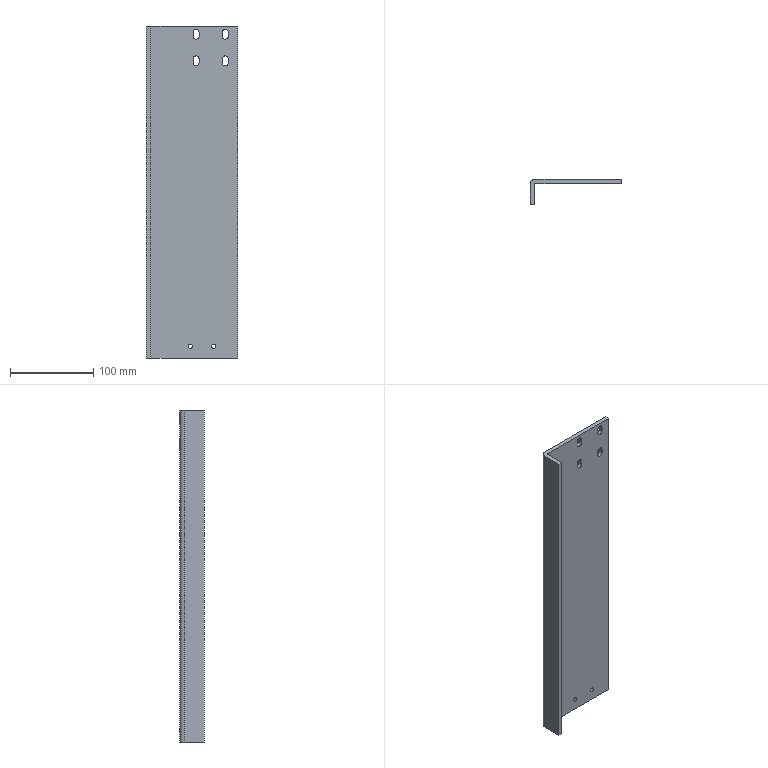Part | STEP file | Hydraulic Cylinder Bracket | 1 solid | 34 faces | box 110 x 30 x 400 mm | volume 265743 mm3 | cylinder 18 | plane 16 | commonest cylinder face diameters 7 x12 5.2 x4 1 x1 11 x1
STEP:
#1=CARTESIAN_POINT('',(81.,20.,16.6));
#2=VERTEX_POINT('',#1);
#3=CARTESIAN_POINT('',(81.,20.,11.4));
#4=VERTEX_POINT('',#3);
#5=CARTESIAN_POINT('',(81.,20.,14.));
#6=DIRECTION('',(0.,-1.,0.));
#7=DIRECTION('',(0.,0.,-1.));
#8=AXIS2_PLACEMENT_3D('',#5,#6,#7);
#9=CIRCLE('',#8,2.6);
#10=EDGE_CURVE('',#2,#4,#9,.T.);
#11=ORIENTED_EDGE('',*,*,#10,.F.);
#12=CARTESIAN_POINT('',(81.,15.,16.6));
#13=VERTEX_POINT('',#12);
#14=CARTESIAN_POINT('',(81.,20.,16.6));
#15=DIRECTION('',(0.,-1.,0.));
#16=VECTOR('',#15,1000.);
#17=LINE('',#14,#16);
#18=EDGE_CURVE('',#2,#13,#17,.T.);
#19=ORIENTED_EDGE('',*,*,#18,.T.);
#20=CARTESIAN_POINT('',(81.,15.,11.4));
#21=VERTEX_POINT('',#20);
#22=CARTESIAN_POINT('',(81.,15.,14.));
#23=DIRECTION('',(0.,1.,0.));
#24=DIRECTION('',(0.,0.,-1.));
#25=AXIS2_PLACEMENT_3D('',#22,#23,#24);
#26=CIRCLE('',#25,2.6);
#27=EDGE_CURVE('',#21,#13,#26,.T.);
#28=ORIENTED_EDGE('',*,*,#27,.F.);
#29=CARTESIAN_POINT('',(81.,20.,11.4));
#30=DIRECTION('',(0.,-1.,0.));
#31=VECTOR('',#30,1000.);
#32=LINE('',#29,#31);
#33=EDGE_CURVE('',#4,#21,#32,.T.);
#34=ORIENTED_EDGE('',*,*,#33,.F.);
#35=EDGE_LOOP('',(#11,#19,#28,#34));
#36=FACE_OUTER_BOUND('',#35,.T.);
#37=CARTESIAN_POINT('',(81.,20.,14.));
#38=DIRECTION('',(0.,-1.,0.));
#39=DIRECTION('',(0.,0.,-1.));
#40=AXIS2_PLACEMENT_3D('',#37,#38,#39);
#41=CYLINDRICAL_SURFACE('',#40,2.6);
#42=ADVANCED_FACE('',(#36),#41,.F.);
#43=CARTESIAN_POINT('',(53.,20.,16.6));
#44=VERTEX_POINT('',#43);
#45=CARTESIAN_POINT('',(53.,20.,11.4));
#46=VERTEX_POINT('',#45);
#47=CARTESIAN_POINT('',(53.,20.,14.));
#48=DIRECTION('',(0.,-1.,0.));
#49=DIRECTION('',(0.,0.,-1.));
#50=AXIS2_PLACEMENT_3D('',#47,#48,#49);
#51=CIRCLE('',#50,2.6);
#52=EDGE_CURVE('',#44,#46,#51,.T.);
#53=ORIENTED_EDGE('',*,*,#52,.F.);
#54=CARTESIAN_POINT('',(53.,15.,16.6));
#55=VERTEX_POINT('',#54);
#56=CARTESIAN_POINT('',(53.,20.,16.6));
#57=DIRECTION('',(0.,-1.,0.));
#58=VECTOR('',#57,1000.);
#59=LINE('',#56,#58);
#60=EDGE_CURVE('',#44,#55,#59,.T.);
#61=ORIENTED_EDGE('',*,*,#60,.T.);
#62=CARTESIAN_POINT('',(53.,15.,11.4));
#63=VERTEX_POINT('',#62);
#64=CARTESIAN_POINT('',(53.,15.,14.));
#65=DIRECTION('',(0.,1.,0.));
#66=DIRECTION('',(0.,0.,-1.));
#67=AXIS2_PLACEMENT_3D('',#64,#65,#66);
#68=CIRCLE('',#67,2.6);
#69=EDGE_CURVE('',#63,#55,#68,.T.);
#70=ORIENTED_EDGE('',*,*,#69,.F.);
#71=CARTESIAN_POINT('',(53.,20.,11.4));
#72=DIRECTION('',(0.,-1.,0.));
#73=VECTOR('',#72,1000.);
#74=LINE('',#71,#73);
#75=EDGE_CURVE('',#46,#63,#74,.T.);
#76=ORIENTED_EDGE('',*,*,#75,.F.);
#77=EDGE_LOOP('',(#53,#61,#70,#76));
#78=FACE_OUTER_BOUND('',#77,.T.);
#79=CARTESIAN_POINT('',(53.,20.,14.));
#80=DIRECTION('',(0.,-1.,0.));
#81=DIRECTION('',(0.,0.,-1.));
#82=AXIS2_PLACEMENT_3D('',#79,#80,#81);
#83=CYLINDRICAL_SURFACE('',#82,2.6);
#84=ADVANCED_FACE('',(#78),#83,.F.);
#85=CARTESIAN_POINT('',(95.,20.,384.));
#86=VERTEX_POINT('',#85);
#87=CARTESIAN_POINT('',(98.5,20.,387.5));
#88=VERTEX_POINT('',#87);
#89=CARTESIAN_POINT('',(95.,20.,387.5));
#90=DIRECTION('',(0.,-1.,0.));
#91=DIRECTION('',(0.,0.,-1.));
#92=AXIS2_PLACEMENT_3D('',#89,#90,#91);
#93=CIRCLE('',#92,3.5);
#94=EDGE_CURVE('',#86,#88,#93,.T.);
#95=ORIENTED_EDGE('',*,*,#94,.F.);
#96=CARTESIAN_POINT('',(95.,15.,384.));
#97=VERTEX_POINT('',#96);
#98=CARTESIAN_POINT('',(95.,25.,384.));
#99=DIRECTION('',(0.,-1.,0.));
#100=VECTOR('',#99,1000.);
#101=LINE('',#98,#100);
#102=EDGE_CURVE('',#86,#97,#101,.T.);
#103=ORIENTED_EDGE('',*,*,#102,.T.);
#104=CARTESIAN_POINT('',(98.5,15.,387.5));
#105=VERTEX_POINT('',#104);
#106=CARTESIAN_POINT('',(95.,15.,387.5));
#107=DIRECTION('',(0.,1.,0.));
#108=DIRECTION('',(0.,0.,-1.));
#109=AXIS2_PLACEMENT_3D('',#106,#107,#108);
#110=CIRCLE('',#109,3.5);
#111=EDGE_CURVE('',#105,#97,#110,.T.);
#112=ORIENTED_EDGE('',*,*,#111,.F.);
#113=CARTESIAN_POINT('',(98.5,25.,387.5));
#114=DIRECTION('',(0.,1.,0.));
#115=VECTOR('',#114,1000.);
#116=LINE('',#113,#115);
#117=EDGE_CURVE('',#105,#88,#116,.T.);
#118=ORIENTED_EDGE('',*,*,#117,.T.);
#119=EDGE_LOOP('',(#95,#103,#112,#118));
#120=FACE_OUTER_BOUND('',#119,.T.);
#121=CARTESIAN_POINT('',(95.,25.,387.5));
#122=DIRECTION('',(0.,-1.,0.));
#123=DIRECTION('',(0.,0.,-1.));
#124=AXIS2_PLACEMENT_3D('',#121,#122,#123);
#125=CYLINDRICAL_SURFACE('',#124,3.5);
#126=ADVANCED_FACE('',(#120),#125,.F.);
#127=CARTESIAN_POINT('',(60.,20.,384.));
#128=VERTEX_POINT('',#127);
#129=CARTESIAN_POINT('',(63.5,20.,387.5));
#130=VERTEX_POINT('',#129);
#131=CARTESIAN_POINT('',(60.,20.,387.5));
#132=DIRECTION('',(0.,-1.,0.));
#133=DIRECTION('',(0.,0.,-1.));
#134=AXIS2_PLACEMENT_3D('',#131,#132,#133);
#135=CIRCLE('',#134,3.5);
#136=EDGE_CURVE('',#128,#130,#135,.T.);
#137=ORIENTED_EDGE('',*,*,#136,.F.);
#138=CARTESIAN_POINT('',(60.,15.,384.));
#139=VERTEX_POINT('',#138);
#140=CARTESIAN_POINT('',(60.,25.,384.));
#141=DIRECTION('',(0.,-1.,0.));
#142=VECTOR('',#141,1000.);
#143=LINE('',#140,#142);
#144=EDGE_CURVE('',#128,#139,#143,.T.);
#145=ORIENTED_EDGE('',*,*,#144,.T.);
#146=CARTESIAN_POINT('',(63.5,15.,387.5));
#147=VERTEX_POINT('',#146);
#148=CARTESIAN_POINT('',(60.,15.,387.5));
#149=DIRECTION('',(0.,1.,0.));
#150=DIRECTION('',(0.,0.,-1.));
#151=AXIS2_PLACEMENT_3D('',#148,#149,#150);
#152=CIRCLE('',#151,3.5);
#153=EDGE_CURVE('',#147,#139,#152,.T.);
#154=ORIENTED_EDGE('',*,*,#153,.F.);
#155=CARTESIAN_POINT('',(63.5,25.,387.5));
#156=DIRECTION('',(0.,1.,0.));
#157=VECTOR('',#156,1000.);
#158=LINE('',#155,#157);
#159=EDGE_CURVE('',#147,#130,#158,.T.);
#160=ORIENTED_EDGE('',*,*,#159,.T.);
#161=EDGE_LOOP('',(#137,#145,#154,#160));
#162=FACE_OUTER_BOUND('',#161,.T.);
#163=CARTESIAN_POINT('',(60.,25.,387.5));
#164=DIRECTION('',(0.,-1.,0.));
#165=DIRECTION('',(0.,0.,-1.));
#166=AXIS2_PLACEMENT_3D('',#163,#164,#165);
#167=CYLINDRICAL_SURFACE('',#166,3.5);
#168=ADVANCED_FACE('',(#162),#167,.F.);
#169=CARTESIAN_POINT('',(60.,20.,352.));
#170=VERTEX_POINT('',#169);
#171=CARTESIAN_POINT('',(63.5,20.,355.5));
#172=VERTEX_POINT('',#171);
#173=CARTESIAN_POINT('',(60.,20.,355.5));
#174=DIRECTION('',(0.,-1.,0.));
#175=DIRECTION('',(0.,0.,-1.));
#176=AXIS2_PLACEMENT_3D('',#173,#174,#175);
#177=CIRCLE('',#176,3.5);
#178=EDGE_CURVE('',#170,#172,#177,.T.);
#179=ORIENTED_EDGE('',*,*,#178,.F.);
#180=CARTESIAN_POINT('',(60.,15.,352.));
#181=VERTEX_POINT('',#180);
#182=CARTESIAN_POINT('',(60.,25.,352.));
#183=DIRECTION('',(0.,-1.,0.));
#184=VECTOR('',#183,1000.);
#185=LINE('',#182,#184);
#186=EDGE_CURVE('',#170,#181,#185,.T.);
#187=ORIENTED_EDGE('',*,*,#186,.T.);
#188=CARTESIAN_POINT('',(63.5,15.,355.5));
#189=VERTEX_POINT('',#188);
#190=CARTESIAN_POINT('',(60.,15.,355.5));
#191=DIRECTION('',(0.,1.,0.));
#192=DIRECTION('',(0.,0.,-1.));
#193=AXIS2_PLACEMENT_3D('',#190,#191,#192);
#194=CIRCLE('',#193,3.5);
#195=EDGE_CURVE('',#189,#181,#194,.T.);
#196=ORIENTED_EDGE('',*,*,#195,.F.);
#197=CARTESIAN_POINT('',(63.5,25.,355.5));
#198=DIRECTION('',(0.,1.,0.));
#199=VECTOR('',#198,1000.);
#200=LINE('',#197,#199);
#201=EDGE_CURVE('',#189,#172,#200,.T.);
#202=ORIENTED_EDGE('',*,*,#201,.T.);
#203=EDGE_LOOP('',(#179,#187,#196,#202));
#204=FACE_OUTER_BOUND('',#203,.T.);
#205=CARTESIAN_POINT('',(60.,25.,355.5));
#206=DIRECTION('',(0.,-1.,0.));
#207=DIRECTION('',(0.,0.,-1.));
#208=AXIS2_PLACEMENT_3D('',#205,#206,#207);
#209=CYLINDRICAL_SURFACE('',#208,3.5);
#210=ADVANCED_FACE('',(#204),#209,.F.);
#211=CARTESIAN_POINT('',(95.,20.,352.));
#212=VERTEX_POINT('',#211);
#213=CARTESIAN_POINT('',(98.5,20.,355.5));
#214=VERTEX_POINT('',#213);
#215=CARTESIAN_POINT('',(95.,20.,355.5));
#216=DIRECTION('',(0.,-1.,0.));
#217=DIRECTION('',(0.,0.,-1.));
#218=AXIS2_PLACEMENT_3D('',#215,#216,#217);
#219=CIRCLE('',#218,3.5);
#220=EDGE_CURVE('',#212,#214,#219,.T.);
#221=ORIENTED_EDGE('',*,*,#220,.F.);
#222=CARTESIAN_POINT('',(95.,15.,352.));
#223=VERTEX_POINT('',#222);
#224=CARTESIAN_POINT('',(95.,25.,352.));
#225=DIRECTION('',(0.,-1.,0.));
#226=VECTOR('',#225,1000.);
#227=LINE('',#224,#226);
#228=EDGE_CURVE('',#212,#223,#227,.T.);
#229=ORIENTED_EDGE('',*,*,#228,.T.);
#230=CARTESIAN_POINT('',(98.5,15.,355.5));
#231=VERTEX_POINT('',#230);
#232=CARTESIAN_POINT('',(95.,15.,355.5));
#233=DIRECTION('',(0.,1.,0.));
#234=DIRECTION('',(0.,0.,-1.));
#235=AXIS2_PLACEMENT_3D('',#232,#233,#234);
#236=CIRCLE('',#235,3.5);
#237=EDGE_CURVE('',#231,#223,#236,.T.);
#238=ORIENTED_EDGE('',*,*,#237,.F.);
#239=CARTESIAN_POINT('',(98.5,25.,355.5));
#240=DIRECTION('',(0.,1.,0.));
#241=VECTOR('',#240,1000.);
#242=LINE('',#239,#241);
#243=EDGE_CURVE('',#231,#214,#242,.T.);
#244=ORIENTED_EDGE('',*,*,#243,.T.);
#245=EDGE_LOOP('',(#221,#229,#238,#244));
#246=FACE_OUTER_BOUND('',#245,.T.);
#247=CARTESIAN_POINT('',(95.,25.,355.5));
#248=DIRECTION('',(0.,-1.,0.));
#249=DIRECTION('',(0.,0.,-1.));
#250=AXIS2_PLACEMENT_3D('',#247,#248,#249);
#251=CYLINDRICAL_SURFACE('',#250,3.5);
#252=ADVANCED_FACE('',(#246),#251,.F.);
#253=CARTESIAN_POINT('',(5.5,20.,400.));
#254=VERTEX_POINT('',#253);
#255=CARTESIAN_POINT('',(110.,20.,400.));
#256=VERTEX_POINT('',#255);
#257=CARTESIAN_POINT('',(0.,20.,400.));
#258=DIRECTION('',(1.,0.,0.));
#259=VECTOR('',#258,1000.);
#260=LINE('',#257,#259);
#261=EDGE_CURVE('',#254,#256,#260,.T.);
#262=ORIENTED_EDGE('',*,*,#261,.T.);
#263=CARTESIAN_POINT('',(110.,20.,0.));
#264=VERTEX_POINT('',#263);
#265=CARTESIAN_POINT('',(110.,20.,400.));
#266=DIRECTION('',(0.,0.,-1.));
#267=VECTOR('',#266,1000.);
#268=LINE('',#265,#267);
#269=EDGE_CURVE('',#256,#264,#268,.T.);
#270=ORIENTED_EDGE('',*,*,#269,.T.);
#271=CARTESIAN_POINT('',(5.5,20.,0.));
#272=VERTEX_POINT('',#271);
#273=CARTESIAN_POINT('',(0.,20.,0.));
#274=DIRECTION('',(-1.,0.,0.));
#275=VECTOR('',#274,1000.);
#276=LINE('',#273,#275);
#277=EDGE_CURVE('',#264,#272,#276,.T.);
#278=ORIENTED_EDGE('',*,*,#277,.T.);
#279=CARTESIAN_POINT('',(5.5,20.,400.));
#280=DIRECTION('',(0.,0.,1.));
#281=VECTOR('',#280,1000.);
#282=LINE('',#279,#281);
#283=EDGE_CURVE('',#272,#254,#282,.T.);
#284=ORIENTED_EDGE('',*,*,#283,.T.);
#285=EDGE_LOOP('',(#262,#270,#278,#284));
#286=FACE_OUTER_BOUND('',#285,.T.);
#287=CARTESIAN_POINT('',(81.,20.,14.));
#288=DIRECTION('',(0.,-1.,0.));
#289=DIRECTION('',(0.,0.,-1.));
#290=AXIS2_PLACEMENT_3D('',#287,#288,#289);
#291=CIRCLE('',#290,2.6);
#292=EDGE_CURVE('',#4,#2,#291,.T.);
#293=ORIENTED_EDGE('',*,*,#292,.T.);
#294=ORIENTED_EDGE('',*,*,#10,.T.);
#295=EDGE_LOOP('',(#293,#294));
#296=FACE_BOUND('',#295,.T.);
#297=CARTESIAN_POINT('',(53.,20.,14.));
#298=DIRECTION('',(0.,-1.,0.));
#299=DIRECTION('',(0.,0.,-1.));
#300=AXIS2_PLACEMENT_3D('',#297,#298,#299);
#301=CIRCLE('',#300,2.6);
#302=EDGE_CURVE('',#46,#44,#301,.T.);
#303=ORIENTED_EDGE('',*,*,#302,.T.);
#304=ORIENTED_EDGE('',*,*,#52,.T.);
#305=EDGE_LOOP('',(#303,#304));
#306=FACE_BOUND('',#305,.T.);
#307=CARTESIAN_POINT('',(91.5,20.,387.5));
#308=VERTEX_POINT('',#307);
#309=CARTESIAN_POINT('',(95.,20.,387.5));
#310=DIRECTION('',(0.,-1.,0.));
#311=DIRECTION('',(0.,0.,-1.));
#312=AXIS2_PLACEMENT_3D('',#309,#310,#311);
#313=CIRCLE('',#312,3.5);
#314=EDGE_CURVE('',#308,#86,#313,.T.);
#315=ORIENTED_EDGE('',*,*,#314,.T.);
#316=ORIENTED_EDGE('',*,*,#94,.T.);
#317=CARTESIAN_POINT('',(98.5,20.,392.5));
#318=VERTEX_POINT('',#317);
#319=CARTESIAN_POINT('',(98.5,20.,400.));
#320=DIRECTION('',(0.,0.,1.));
#321=VECTOR('',#320,1000.);
#322=LINE('',#319,#321);
#323=EDGE_CURVE('',#88,#318,#322,.T.);
#324=ORIENTED_EDGE('',*,*,#323,.T.);
#325=CARTESIAN_POINT('',(91.5,20.,392.5));
#326=VERTEX_POINT('',#325);
#327=CARTESIAN_POINT('',(95.,20.,392.5));
#328=DIRECTION('',(0.,-1.,0.));
#329=DIRECTION('',(0.,0.,-1.));
#330=AXIS2_PLACEMENT_3D('',#327,#328,#329);
#331=CIRCLE('',#330,3.5);
#332=EDGE_CURVE('',#318,#326,#331,.T.);
#333=ORIENTED_EDGE('',*,*,#332,.T.);
#334=CARTESIAN_POINT('',(91.5,20.,400.));
#335=DIRECTION('',(0.,0.,-1.));
#336=VECTOR('',#335,1000.);
#337=LINE('',#334,#336);
#338=EDGE_CURVE('',#326,#308,#337,.T.);
#339=ORIENTED_EDGE('',*,*,#338,.T.);
#340=EDGE_LOOP('',(#315,#316,#324,#333,#339));
#341=FACE_BOUND('',#340,.T.);
#342=CARTESIAN_POINT('',(56.5,20.,387.5));
#343=VERTEX_POINT('',#342);
#344=CARTESIAN_POINT('',(60.,20.,387.5));
#345=DIRECTION('',(0.,-1.,0.));
#346=DIRECTION('',(0.,0.,-1.));
#347=AXIS2_PLACEMENT_3D('',#344,#345,#346);
#348=CIRCLE('',#347,3.5);
#349=EDGE_CURVE('',#343,#128,#348,.T.);
#350=ORIENTED_EDGE('',*,*,#349,.T.);
#351=ORIENTED_EDGE('',*,*,#136,.T.);
#352=CARTESIAN_POINT('',(63.5,20.,392.5));
#353=VERTEX_POINT('',#352);
#354=CARTESIAN_POINT('',(63.5,20.,400.));
#355=DIRECTION('',(0.,0.,1.));
#356=VECTOR('',#355,1000.);
#357=LINE('',#354,#356);
#358=EDGE_CURVE('',#130,#353,#357,.T.);
#359=ORIENTED_EDGE('',*,*,#358,.T.);
#360=CARTESIAN_POINT('',(56.5,20.,392.5));
#361=VERTEX_POINT('',#360);
#362=CARTESIAN_POINT('',(60.,20.,392.5));
#363=DIRECTION('',(0.,-1.,0.));
#364=DIRECTION('',(0.,0.,-1.));
#365=AXIS2_PLACEMENT_3D('',#362,#363,#364);
#366=CIRCLE('',#365,3.5);
#367=EDGE_CURVE('',#353,#361,#366,.T.);
#368=ORIENTED_EDGE('',*,*,#367,.T.);
#369=CARTESIAN_POINT('',(56.5,20.,400.));
#370=DIRECTION('',(0.,0.,-1.));
#371=VECTOR('',#370,1000.);
#372=LINE('',#369,#371);
#373=EDGE_CURVE('',#361,#343,#372,.T.);
#374=ORIENTED_EDGE('',*,*,#373,.T.);
#375=EDGE_LOOP('',(#350,#351,#359,#368,#374));
#376=FACE_BOUND('',#375,.T.);
#377=CARTESIAN_POINT('',(56.5,20.,360.5));
#378=VERTEX_POINT('',#377);
#379=CARTESIAN_POINT('',(56.5,20.,355.5));
#380=VERTEX_POINT('',#379);
#381=CARTESIAN_POINT('',(56.5,20.,400.));
#382=DIRECTION('',(0.,0.,-1.));
#383=VECTOR('',#382,1000.);
#384=LINE('',#381,#383);
#385=EDGE_CURVE('',#378,#380,#384,.T.);
#386=ORIENTED_EDGE('',*,*,#385,.T.);
#387=CARTESIAN_POINT('',(60.,20.,355.5));
#388=DIRECTION('',(0.,-1.,0.));
#389=DIRECTION('',(0.,0.,-1.));
#390=AXIS2_PLACEMENT_3D('',#387,#388,#389);
#391=CIRCLE('',#390,3.5);
#392=EDGE_CURVE('',#380,#170,#391,.T.);
#393=ORIENTED_EDGE('',*,*,#392,.T.);
#394=ORIENTED_EDGE('',*,*,#178,.T.);
#395=CARTESIAN_POINT('',(63.5,20.,360.5));
#396=VERTEX_POINT('',#395);
#397=CARTESIAN_POINT('',(63.5,20.,400.));
#398=DIRECTION('',(0.,0.,1.));
#399=VECTOR('',#398,1000.);
#400=LINE('',#397,#399);
#401=EDGE_CURVE('',#172,#396,#400,.T.);
#402=ORIENTED_EDGE('',*,*,#401,.T.);
#403=CARTESIAN_POINT('',(60.,20.,360.5));
#404=DIRECTION('',(0.,-1.,0.));
#405=DIRECTION('',(0.,0.,-1.));
#406=AXIS2_PLACEMENT_3D('',#403,#404,#405);
#407=CIRCLE('',#406,3.5);
#408=EDGE_CURVE('',#396,#378,#407,.T.);
#409=ORIENTED_EDGE('',*,*,#408,.T.);
#410=EDGE_LOOP('',(#386,#393,#394,#402,#409));
#411=FACE_BOUND('',#410,.T.);
#412=CARTESIAN_POINT('',(91.5,20.,360.5));
#413=VERTEX_POINT('',#412);
#414=CARTESIAN_POINT('',(91.5,20.,355.5));
#415=VERTEX_POINT('',#414);
#416=CARTESIAN_POINT('',(91.5,20.,400.));
#417=DIRECTION('',(0.,0.,-1.));
#418=VECTOR('',#417,1000.);
#419=LINE('',#416,#418);
#420=EDGE_CURVE('',#413,#415,#419,.T.);
#421=ORIENTED_EDGE('',*,*,#420,.T.);
#422=CARTESIAN_POINT('',(95.,20.,355.5));
#423=DIRECTION('',(0.,-1.,0.));
#424=DIRECTION('',(0.,0.,-1.));
#425=AXIS2_PLACEMENT_3D('',#422,#423,#424);
#426=CIRCLE('',#425,3.5);
#427=EDGE_CURVE('',#415,#212,#426,.T.);
#428=ORIENTED_EDGE('',*,*,#427,.T.);
#429=ORIENTED_EDGE('',*,*,#220,.T.);
#430=CARTESIAN_POINT('',(98.5,20.,360.5));
#431=VERTEX_POINT('',#430);
#432=CARTESIAN_POINT('',(98.5,20.,400.));
#433=DIRECTION('',(0.,0.,1.));
#434=VECTOR('',#433,1000.);
#435=LINE('',#432,#434);
#436=EDGE_CURVE('',#214,#431,#435,.T.);
#437=ORIENTED_EDGE('',*,*,#436,.T.);
#438=CARTESIAN_POINT('',(95.,20.,360.5));
#439=DIRECTION('',(0.,-1.,0.));
#440=DIRECTION('',(0.,0.,-1.));
#441=AXIS2_PLACEMENT_3D('',#438,#439,#440);
#442=CIRCLE('',#441,3.5);
#443=EDGE_CURVE('',#431,#413,#442,.T.);
#444=ORIENTED_EDGE('',*,*,#443,.T.);
#445=EDGE_LOOP('',(#421,#428,#429,#437,#444));
#446=FACE_BOUND('',#445,.T.);
#447=CARTESIAN_POINT('',(0.,20.,400.));
#448=DIRECTION('',(0.,1.,0.));
#449=DIRECTION('',(0.,0.,1.));
#450=AXIS2_PLACEMENT_3D('',#447,#448,#449);
#451=PLANE('',#450);
#452=ADVANCED_FACE('',(#286,#296,#306,#341,#376,#411,#446),#451,.T.);
#453=CARTESIAN_POINT('',(110.,15.,400.));
#454=VERTEX_POINT('',#453);
#455=CARTESIAN_POINT('',(110.,20.,400.));
#456=DIRECTION('',(0.,-1.,0.));
#457=VECTOR('',#456,1000.);
#458=LINE('',#455,#457);
#459=EDGE_CURVE('',#256,#454,#458,.T.);
#460=ORIENTED_EDGE('',*,*,#459,.T.);
#461=CARTESIAN_POINT('',(110.,15.,0.));
#462=VERTEX_POINT('',#461);
#463=CARTESIAN_POINT('',(110.,15.,400.));
#464=DIRECTION('',(0.,0.,-1.));
#465=VECTOR('',#464,1000.);
#466=LINE('',#463,#465);
#467=EDGE_CURVE('',#454,#462,#466,.T.);
#468=ORIENTED_EDGE('',*,*,#467,.T.);
#469=CARTESIAN_POINT('',(110.,20.,0.));
#470=DIRECTION('',(0.,1.,0.));
#471=VECTOR('',#470,1000.);
#472=LINE('',#469,#471);
#473=EDGE_CURVE('',#462,#264,#472,.T.);
#474=ORIENTED_EDGE('',*,*,#473,.T.);
#475=ORIENTED_EDGE('',*,*,#269,.F.);
#476=EDGE_LOOP('',(#460,#468,#474,#475));
#477=FACE_OUTER_BOUND('',#476,.T.);
#478=CARTESIAN_POINT('',(110.,20.,400.));
#479=DIRECTION('',(1.,0.,0.));
#480=DIRECTION('',(0.,0.,-1.));
#481=AXIS2_PLACEMENT_3D('',#478,#479,#480);
#482=PLANE('',#481);
#483=ADVANCED_FACE('',(#477),#482,.T.);
#484=CARTESIAN_POINT('',(5.5,15.,400.));
#485=VERTEX_POINT('',#484);
#486=CARTESIAN_POINT('',(0.,15.,400.));
#487=DIRECTION('',(-1.,0.,0.));
#488=VECTOR('',#487,1000.);
#489=LINE('',#486,#488);
#490=EDGE_CURVE('',#454,#485,#489,.T.);
#491=ORIENTED_EDGE('',*,*,#490,.F.);
#492=ORIENTED_EDGE('',*,*,#459,.F.);
#493=ORIENTED_EDGE('',*,*,#261,.F.);
#494=CARTESIAN_POINT('',(0.,14.5,400.));
#495=VERTEX_POINT('',#494);
#496=CARTESIAN_POINT('',(5.5,14.5,400.));
#497=DIRECTION('',(0.,0.,-1.));
#498=DIRECTION('',(-1.,0.,0.));
#499=AXIS2_PLACEMENT_3D('',#496,#497,#498);
#500=CIRCLE('',#499,5.5);
#501=EDGE_CURVE('',#495,#254,#500,.T.);
#502=ORIENTED_EDGE('',*,*,#501,.F.);
#503=CARTESIAN_POINT('',(0.,-10.,400.));
#504=VERTEX_POINT('',#503);
#505=CARTESIAN_POINT('',(0.,0.,400.));
#506=DIRECTION('',(0.,1.,0.));
#507=VECTOR('',#506,1000.);
#508=LINE('',#505,#507);
#509=EDGE_CURVE('',#504,#495,#508,.T.);
#510=ORIENTED_EDGE('',*,*,#509,.F.);
#511=CARTESIAN_POINT('',(5.,-10.,400.));
#512=VERTEX_POINT('',#511);
#513=CARTESIAN_POINT('',(0.,-10.,400.));
#514=DIRECTION('',(1.,0.,0.));
#515=VECTOR('',#514,1000.);
#516=LINE('',#513,#515);
#517=EDGE_CURVE('',#504,#512,#516,.T.);
#518=ORIENTED_EDGE('',*,*,#517,.T.);
#519=CARTESIAN_POINT('',(5.,14.5,400.));
#520=VERTEX_POINT('',#519);
#521=CARTESIAN_POINT('',(5.,-10.,400.));
#522=DIRECTION('',(0.,1.,0.));
#523=VECTOR('',#522,1000.);
#524=LINE('',#521,#523);
#525=EDGE_CURVE('',#512,#520,#524,.T.);
#526=ORIENTED_EDGE('',*,*,#525,.T.);
#527=CARTESIAN_POINT('',(5.5,14.5,400.));
#528=DIRECTION('',(0.,0.,-1.));
#529=DIRECTION('',(-1.,0.,0.));
#530=AXIS2_PLACEMENT_3D('',#527,#528,#529);
#531=CIRCLE('',#530,0.5);
#532=EDGE_CURVE('',#520,#485,#531,.T.);
#533=ORIENTED_EDGE('',*,*,#532,.T.);
#534=EDGE_LOOP('',(#491,#492,#493,#502,#510,#518,#526,#533));
#535=FACE_OUTER_BOUND('',#534,.T.);
#536=CARTESIAN_POINT('',(0.,0.,400.));
#537=DIRECTION('',(0.,0.,-1.));
#538=DIRECTION('',(-1.,0.,0.));
#539=AXIS2_PLACEMENT_3D('',#536,#537,#538);
#540=PLANE('',#539);
#541=ADVANCED_FACE('',(#535),#540,.F.);
#542=CARTESIAN_POINT('',(0.,14.5,0.));
#543=VERTEX_POINT('',#542);
#544=CARTESIAN_POINT('',(0.,14.5,0.));
#545=DIRECTION('',(0.,0.,1.));
#546=VECTOR('',#545,1000.);
#547=LINE('',#544,#546);
#548=EDGE_CURVE('',#543,#495,#547,.T.);
#549=ORIENTED_EDGE('',*,*,#548,.T.);
#550=ORIENTED_EDGE('',*,*,#501,.T.);
#551=ORIENTED_EDGE('',*,*,#283,.F.);
#552=CARTESIAN_POINT('',(5.5,14.5,0.));
#553=DIRECTION('',(0.,0.,1.));
#554=DIRECTION('',(-1.,0.,0.));
#555=AXIS2_PLACEMENT_3D('',#552,#553,#554);
#556=CIRCLE('',#555,5.5);
#557=EDGE_CURVE('',#272,#543,#556,.T.);
#558=ORIENTED_EDGE('',*,*,#557,.T.);
#559=EDGE_LOOP('',(#549,#550,#551,#558));
#560=FACE_OUTER_BOUND('',#559,.T.);
#561=CARTESIAN_POINT('',(5.5,14.5,0.));
#562=DIRECTION('',(0.,0.,-1.));
#563=DIRECTION('',(-1.,0.,0.));
#564=AXIS2_PLACEMENT_3D('',#561,#562,#563);
#565=CYLINDRICAL_SURFACE('',#564,5.5);
#566=ADVANCED_FACE('',(#560),#565,.T.);
#567=ORIENTED_EDGE('',*,*,#277,.F.);
#568=ORIENTED_EDGE('',*,*,#473,.F.);
#569=CARTESIAN_POINT('',(5.5,15.,0.));
#570=VERTEX_POINT('',#569);
#571=CARTESIAN_POINT('',(0.,15.,0.));
#572=DIRECTION('',(-1.,0.,0.));
#573=VECTOR('',#572,1000.);
#574=LINE('',#571,#573);
#575=EDGE_CURVE('',#462,#570,#574,.T.);
#576=ORIENTED_EDGE('',*,*,#575,.T.);
#577=CARTESIAN_POINT('',(5.,14.5,0.));
#578=VERTEX_POINT('',#577);
#579=CARTESIAN_POINT('',(5.5,14.5,0.));
#580=DIRECTION('',(0.,0.,-1.));
#581=DIRECTION('',(-1.,0.,0.));
#582=AXIS2_PLACEMENT_3D('',#579,#580,#581);
#583=CIRCLE('',#582,0.5);
#584=EDGE_CURVE('',#578,#570,#583,.T.);
#585=ORIENTED_EDGE('',*,*,#584,.F.);
#586=CARTESIAN_POINT('',(5.,-10.,0.));
#587=VERTEX_POINT('',#586);
#588=CARTESIAN_POINT('',(5.,15.,0.));
#589=DIRECTION('',(0.,-1.,0.));
#590=VECTOR('',#589,1000.);
#591=LINE('',#588,#590);
#592=EDGE_CURVE('',#578,#587,#591,.T.);
#593=ORIENTED_EDGE('',*,*,#592,.T.);
#594=CARTESIAN_POINT('',(0.,-10.,0.));
#595=VERTEX_POINT('',#594);
#596=CARTESIAN_POINT('',(0.,-10.,0.));
#597=DIRECTION('',(1.,0.,0.));
#598=VECTOR('',#597,1000.);
#599=LINE('',#596,#598);
#600=EDGE_CURVE('',#595,#587,#599,.T.);
#601=ORIENTED_EDGE('',*,*,#600,.F.);
#602=CARTESIAN_POINT('',(0.,0.,0.));
#603=DIRECTION('',(0.,-1.,0.));
#604=VECTOR('',#603,1000.);
#605=LINE('',#602,#604);
#606=EDGE_CURVE('',#543,#595,#605,.T.);
#607=ORIENTED_EDGE('',*,*,#606,.F.);
#608=ORIENTED_EDGE('',*,*,#557,.F.);
#609=EDGE_LOOP('',(#567,#568,#576,#585,#593,#601,#607,#608));
#610=FACE_OUTER_BOUND('',#609,.T.);
#611=CARTESIAN_POINT('',(0.,0.,0.));
#612=DIRECTION('',(0.,0.,-1.));
#613=DIRECTION('',(-1.,0.,0.));
#614=AXIS2_PLACEMENT_3D('',#611,#612,#613);
#615=PLANE('',#614);
#616=ADVANCED_FACE('',(#610),#615,.T.);
#617=ORIENTED_EDGE('',*,*,#18,.F.);
#618=ORIENTED_EDGE('',*,*,#292,.F.);
#619=ORIENTED_EDGE('',*,*,#33,.T.);
#620=CARTESIAN_POINT('',(81.,15.,14.));
#621=DIRECTION('',(0.,1.,0.));
#622=DIRECTION('',(0.,0.,-1.));
#623=AXIS2_PLACEMENT_3D('',#620,#621,#622);
#624=CIRCLE('',#623,2.6);
#625=EDGE_CURVE('',#13,#21,#624,.T.);
#626=ORIENTED_EDGE('',*,*,#625,.F.);
#627=EDGE_LOOP('',(#617,#618,#619,#626));
#628=FACE_OUTER_BOUND('',#627,.T.);
#629=CARTESIAN_POINT('',(81.,20.,14.));
#630=DIRECTION('',(0.,-1.,0.));
#631=DIRECTION('',(0.,0.,-1.));
#632=AXIS2_PLACEMENT_3D('',#629,#630,#631);
#633=CYLINDRICAL_SURFACE('',#632,2.6);
#634=ADVANCED_FACE('',(#628),#633,.F.);
#635=ORIENTED_EDGE('',*,*,#60,.F.);
#636=ORIENTED_EDGE('',*,*,#302,.F.);
#637=ORIENTED_EDGE('',*,*,#75,.T.);
#638=CARTESIAN_POINT('',(53.,15.,14.));
#639=DIRECTION('',(0.,1.,0.));
#640=DIRECTION('',(0.,0.,-1.));
#641=AXIS2_PLACEMENT_3D('',#638,#639,#640);
#642=CIRCLE('',#641,2.6);
#643=EDGE_CURVE('',#55,#63,#642,.T.);
#644=ORIENTED_EDGE('',*,*,#643,.F.);
#645=EDGE_LOOP('',(#635,#636,#637,#644));
#646=FACE_OUTER_BOUND('',#645,.T.);
#647=CARTESIAN_POINT('',(53.,20.,14.));
#648=DIRECTION('',(0.,-1.,0.));
#649=DIRECTION('',(0.,0.,-1.));
#650=AXIS2_PLACEMENT_3D('',#647,#648,#649);
#651=CYLINDRICAL_SURFACE('',#650,2.6);
#652=ADVANCED_FACE('',(#646),#651,.F.);
#653=ORIENTED_EDGE('',*,*,#117,.F.);
#654=CARTESIAN_POINT('',(98.5,15.,392.5));
#655=VERTEX_POINT('',#654);
#656=CARTESIAN_POINT('',(98.5,15.,392.5));
#657=DIRECTION('',(0.,0.,-1.));
#658=VECTOR('',#657,1000.);
#659=LINE('',#656,#658);
#660=EDGE_CURVE('',#655,#105,#659,.T.);
#661=ORIENTED_EDGE('',*,*,#660,.F.);
#662=CARTESIAN_POINT('',(98.5,25.,392.5));
#663=DIRECTION('',(0.,-1.,0.));
#664=VECTOR('',#663,1000.);
#665=LINE('',#662,#664);
#666=EDGE_CURVE('',#318,#655,#665,.T.);
#667=ORIENTED_EDGE('',*,*,#666,.F.);
#668=ORIENTED_EDGE('',*,*,#323,.F.);
#669=EDGE_LOOP('',(#653,#661,#667,#668));
#670=FACE_OUTER_BOUND('',#669,.T.);
#671=CARTESIAN_POINT('',(98.5,25.,392.5));
#672=DIRECTION('',(1.,0.,0.));
#673=DIRECTION('',(0.,0.,-1.));
#674=AXIS2_PLACEMENT_3D('',#671,#672,#673);
#675=PLANE('',#674);
#676=ADVANCED_FACE('',(#670),#675,.F.);
#677=ORIENTED_EDGE('',*,*,#102,.F.);
#678=ORIENTED_EDGE('',*,*,#314,.F.);
#679=CARTESIAN_POINT('',(91.5,15.,387.5));
#680=VERTEX_POINT('',#679);
#681=CARTESIAN_POINT('',(91.5,25.,387.5));
#682=DIRECTION('',(0.,1.,0.));
#683=VECTOR('',#682,1000.);
#684=LINE('',#681,#683);
#685=EDGE_CURVE('',#680,#308,#684,.T.);
#686=ORIENTED_EDGE('',*,*,#685,.F.);
#687=CARTESIAN_POINT('',(95.,15.,387.5));
#688=DIRECTION('',(0.,1.,0.));
#689=DIRECTION('',(0.,0.,-1.));
#690=AXIS2_PLACEMENT_3D('',#687,#688,#689);
#691=CIRCLE('',#690,3.5);
#692=EDGE_CURVE('',#97,#680,#691,.T.);
#693=ORIENTED_EDGE('',*,*,#692,.F.);
#694=EDGE_LOOP('',(#677,#678,#686,#693));
#695=FACE_OUTER_BOUND('',#694,.T.);
#696=CARTESIAN_POINT('',(95.,25.,387.5));
#697=DIRECTION('',(0.,-1.,0.));
#698=DIRECTION('',(0.,0.,-1.));
#699=AXIS2_PLACEMENT_3D('',#696,#697,#698);
#700=CYLINDRICAL_SURFACE('',#699,3.5);
#701=ADVANCED_FACE('',(#695),#700,.F.);
#702=CARTESIAN_POINT('',(91.5,15.,392.5));
#703=VERTEX_POINT('',#702);
#704=CARTESIAN_POINT('',(91.5,25.,392.5));
#705=DIRECTION('',(0.,1.,0.));
#706=VECTOR('',#705,1000.);
#707=LINE('',#704,#706);
#708=EDGE_CURVE('',#703,#326,#707,.T.);
#709=ORIENTED_EDGE('',*,*,#708,.F.);
#710=CARTESIAN_POINT('',(91.5,15.,392.5));
#711=DIRECTION('',(0.,0.,1.));
#712=VECTOR('',#711,1000.);
#713=LINE('',#710,#712);
#714=EDGE_CURVE('',#680,#703,#713,.T.);
#715=ORIENTED_EDGE('',*,*,#714,.F.);
#716=ORIENTED_EDGE('',*,*,#685,.T.);
#717=ORIENTED_EDGE('',*,*,#338,.F.);
#718=EDGE_LOOP('',(#709,#715,#716,#717));
#719=FACE_OUTER_BOUND('',#718,.T.);
#720=CARTESIAN_POINT('',(91.5,25.,392.5));
#721=DIRECTION('',(-1.,0.,0.));
#722=DIRECTION('',(0.,0.,1.));
#723=AXIS2_PLACEMENT_3D('',#720,#721,#722);
#724=PLANE('',#723);
#725=ADVANCED_FACE('',(#719),#724,.F.);
#726=ORIENTED_EDGE('',*,*,#666,.T.);
#727=CARTESIAN_POINT('',(95.,15.,392.5));
#728=DIRECTION('',(0.,1.,0.));
#729=DIRECTION('',(0.,0.,-1.));
#730=AXIS2_PLACEMENT_3D('',#727,#728,#729);
#731=CIRCLE('',#730,3.5);
#732=EDGE_CURVE('',#703,#655,#731,.T.);
#733=ORIENTED_EDGE('',*,*,#732,.F.);
#734=ORIENTED_EDGE('',*,*,#708,.T.);
#735=ORIENTED_EDGE('',*,*,#332,.F.);
#736=EDGE_LOOP('',(#726,#733,#734,#735));
#737=FACE_OUTER_BOUND('',#736,.T.);
#738=CARTESIAN_POINT('',(95.,25.,392.5));
#739=DIRECTION('',(0.,-1.,0.));
#740=DIRECTION('',(0.,0.,-1.));
#741=AXIS2_PLACEMENT_3D('',#738,#739,#740);
#742=CYLINDRICAL_SURFACE('',#741,3.5);
#743=ADVANCED_FACE('',(#737),#742,.F.);
#744=ORIENTED_EDGE('',*,*,#159,.F.);
#745=CARTESIAN_POINT('',(63.5,15.,392.5));
#746=VERTEX_POINT('',#745);
#747=CARTESIAN_POINT('',(63.5,15.,392.5));
#748=DIRECTION('',(0.,0.,-1.));
#749=VECTOR('',#748,1000.);
#750=LINE('',#747,#749);
#751=EDGE_CURVE('',#746,#147,#750,.T.);
#752=ORIENTED_EDGE('',*,*,#751,.F.);
#753=CARTESIAN_POINT('',(63.5,25.,392.5));
#754=DIRECTION('',(0.,-1.,0.));
#755=VECTOR('',#754,1000.);
#756=LINE('',#753,#755);
#757=EDGE_CURVE('',#353,#746,#756,.T.);
#758=ORIENTED_EDGE('',*,*,#757,.F.);
#759=ORIENTED_EDGE('',*,*,#358,.F.);
#760=EDGE_LOOP('',(#744,#752,#758,#759));
#761=FACE_OUTER_BOUND('',#760,.T.);
#762=CARTESIAN_POINT('',(63.5,25.,392.5));
#763=DIRECTION('',(1.,0.,0.));
#764=DIRECTION('',(0.,0.,-1.));
#765=AXIS2_PLACEMENT_3D('',#762,#763,#764);
#766=PLANE('',#765);
#767=ADVANCED_FACE('',(#761),#766,.F.);
#768=ORIENTED_EDGE('',*,*,#144,.F.);
#769=ORIENTED_EDGE('',*,*,#349,.F.);
#770=CARTESIAN_POINT('',(56.5,15.,387.5));
#771=VERTEX_POINT('',#770);
#772=CARTESIAN_POINT('',(56.5,25.,387.5));
#773=DIRECTION('',(0.,1.,0.));
#774=VECTOR('',#773,1000.);
#775=LINE('',#772,#774);
#776=EDGE_CURVE('',#771,#343,#775,.T.);
#777=ORIENTED_EDGE('',*,*,#776,.F.);
#778=CARTESIAN_POINT('',(60.,15.,387.5));
#779=DIRECTION('',(0.,1.,0.));
#780=DIRECTION('',(0.,0.,-1.));
#781=AXIS2_PLACEMENT_3D('',#778,#779,#780);
#782=CIRCLE('',#781,3.5);
#783=EDGE_CURVE('',#139,#771,#782,.T.);
#784=ORIENTED_EDGE('',*,*,#783,.F.);
#785=EDGE_LOOP('',(#768,#769,#777,#784));
#786=FACE_OUTER_BOUND('',#785,.T.);
#787=CARTESIAN_POINT('',(60.,25.,387.5));
#788=DIRECTION('',(0.,-1.,0.));
#789=DIRECTION('',(0.,0.,-1.));
#790=AXIS2_PLACEMENT_3D('',#787,#788,#789);
#791=CYLINDRICAL_SURFACE('',#790,3.5);
#792=ADVANCED_FACE('',(#786),#791,.F.);
#793=CARTESIAN_POINT('',(56.5,15.,392.5));
#794=VERTEX_POINT('',#793);
#795=CARTESIAN_POINT('',(56.5,25.,392.5));
#796=DIRECTION('',(0.,1.,0.));
#797=VECTOR('',#796,1000.);
#798=LINE('',#795,#797);
#799=EDGE_CURVE('',#794,#361,#798,.T.);
#800=ORIENTED_EDGE('',*,*,#799,.F.);
#801=CARTESIAN_POINT('',(56.5,15.,392.5));
#802=DIRECTION('',(0.,0.,1.));
#803=VECTOR('',#802,1000.);
#804=LINE('',#801,#803);
#805=EDGE_CURVE('',#771,#794,#804,.T.);
#806=ORIENTED_EDGE('',*,*,#805,.F.);
#807=ORIENTED_EDGE('',*,*,#776,.T.);
#808=ORIENTED_EDGE('',*,*,#373,.F.);
#809=EDGE_LOOP('',(#800,#806,#807,#808));
#810=FACE_OUTER_BOUND('',#809,.T.);
#811=CARTESIAN_POINT('',(56.5,25.,392.5));
#812=DIRECTION('',(-1.,0.,0.));
#813=DIRECTION('',(0.,0.,1.));
#814=AXIS2_PLACEMENT_3D('',#811,#812,#813);
#815=PLANE('',#814);
#816=ADVANCED_FACE('',(#810),#815,.F.);
#817=ORIENTED_EDGE('',*,*,#757,.T.);
#818=CARTESIAN_POINT('',(60.,15.,392.5));
#819=DIRECTION('',(0.,1.,0.));
#820=DIRECTION('',(0.,0.,-1.));
#821=AXIS2_PLACEMENT_3D('',#818,#819,#820);
#822=CIRCLE('',#821,3.5);
#823=EDGE_CURVE('',#794,#746,#822,.T.);
#824=ORIENTED_EDGE('',*,*,#823,.F.);
#825=ORIENTED_EDGE('',*,*,#799,.T.);
#826=ORIENTED_EDGE('',*,*,#367,.F.);
#827=EDGE_LOOP('',(#817,#824,#825,#826));
#828=FACE_OUTER_BOUND('',#827,.T.);
#829=CARTESIAN_POINT('',(60.,25.,392.5));
#830=DIRECTION('',(0.,-1.,0.));
#831=DIRECTION('',(0.,0.,-1.));
#832=AXIS2_PLACEMENT_3D('',#829,#830,#831);
#833=CYLINDRICAL_SURFACE('',#832,3.5);
#834=ADVANCED_FACE('',(#828),#833,.F.);
#835=ORIENTED_EDGE('',*,*,#186,.F.);
#836=ORIENTED_EDGE('',*,*,#392,.F.);
#837=CARTESIAN_POINT('',(56.5,15.,355.5));
#838=VERTEX_POINT('',#837);
#839=CARTESIAN_POINT('',(56.5,25.,355.5));
#840=DIRECTION('',(0.,1.,0.));
#841=VECTOR('',#840,1000.);
#842=LINE('',#839,#841);
#843=EDGE_CURVE('',#838,#380,#842,.T.);
#844=ORIENTED_EDGE('',*,*,#843,.F.);
#845=CARTESIAN_POINT('',(60.,15.,355.5));
#846=DIRECTION('',(0.,1.,0.));
#847=DIRECTION('',(0.,0.,-1.));
#848=AXIS2_PLACEMENT_3D('',#845,#846,#847);
#849=CIRCLE('',#848,3.5);
#850=EDGE_CURVE('',#181,#838,#849,.T.);
#851=ORIENTED_EDGE('',*,*,#850,.F.);
#852=EDGE_LOOP('',(#835,#836,#844,#851));
#853=FACE_OUTER_BOUND('',#852,.T.);
#854=CARTESIAN_POINT('',(60.,25.,355.5));
#855=DIRECTION('',(0.,-1.,0.));
#856=DIRECTION('',(0.,0.,-1.));
#857=AXIS2_PLACEMENT_3D('',#854,#855,#856);
#858=CYLINDRICAL_SURFACE('',#857,3.5);
#859=ADVANCED_FACE('',(#853),#858,.F.);
#860=CARTESIAN_POINT('',(56.5,15.,360.5));
#861=VERTEX_POINT('',#860);
#862=CARTESIAN_POINT('',(56.5,25.,360.5));
#863=DIRECTION('',(0.,1.,0.));
#864=VECTOR('',#863,1000.);
#865=LINE('',#862,#864);
#866=EDGE_CURVE('',#861,#378,#865,.T.);
#867=ORIENTED_EDGE('',*,*,#866,.F.);
#868=CARTESIAN_POINT('',(56.5,15.,355.5));
#869=DIRECTION('',(0.,0.,1.));
#870=VECTOR('',#869,1000.);
#871=LINE('',#868,#870);
#872=EDGE_CURVE('',#838,#861,#871,.T.);
#873=ORIENTED_EDGE('',*,*,#872,.F.);
#874=ORIENTED_EDGE('',*,*,#843,.T.);
#875=ORIENTED_EDGE('',*,*,#385,.F.);
#876=EDGE_LOOP('',(#867,#873,#874,#875));
#877=FACE_OUTER_BOUND('',#876,.T.);
#878=CARTESIAN_POINT('',(56.5,25.,355.5));
#879=DIRECTION('',(-1.,0.,0.));
#880=DIRECTION('',(0.,0.,1.));
#881=AXIS2_PLACEMENT_3D('',#878,#879,#880);
#882=PLANE('',#881);
#883=ADVANCED_FACE('',(#877),#882,.F.);
#884=CARTESIAN_POINT('',(63.5,15.,360.5));
#885=VERTEX_POINT('',#884);
#886=CARTESIAN_POINT('',(63.5,25.,360.5));
#887=DIRECTION('',(0.,1.,0.));
#888=VECTOR('',#887,1000.);
#889=LINE('',#886,#888);
#890=EDGE_CURVE('',#885,#396,#889,.T.);
#891=ORIENTED_EDGE('',*,*,#890,.F.);
#892=CARTESIAN_POINT('',(60.,15.,360.5));
#893=DIRECTION('',(0.,1.,0.));
#894=DIRECTION('',(0.,0.,-1.));
#895=AXIS2_PLACEMENT_3D('',#892,#893,#894);
#896=CIRCLE('',#895,3.5);
#897=EDGE_CURVE('',#861,#885,#896,.T.);
#898=ORIENTED_EDGE('',*,*,#897,.F.);
#899=ORIENTED_EDGE('',*,*,#866,.T.);
#900=ORIENTED_EDGE('',*,*,#408,.F.);
#901=EDGE_LOOP('',(#891,#898,#899,#900));
#902=FACE_OUTER_BOUND('',#901,.T.);
#903=CARTESIAN_POINT('',(60.,25.,360.5));
#904=DIRECTION('',(0.,-1.,0.));
#905=DIRECTION('',(0.,0.,-1.));
#906=AXIS2_PLACEMENT_3D('',#903,#904,#905);
#907=CYLINDRICAL_SURFACE('',#906,3.5);
#908=ADVANCED_FACE('',(#902),#907,.F.);
#909=ORIENTED_EDGE('',*,*,#201,.F.);
#910=CARTESIAN_POINT('',(63.5,15.,355.5));
#911=DIRECTION('',(0.,0.,-1.));
#912=VECTOR('',#911,1000.);
#913=LINE('',#910,#912);
#914=EDGE_CURVE('',#885,#189,#913,.T.);
#915=ORIENTED_EDGE('',*,*,#914,.F.);
#916=ORIENTED_EDGE('',*,*,#890,.T.);
#917=ORIENTED_EDGE('',*,*,#401,.F.);
#918=EDGE_LOOP('',(#909,#915,#916,#917));
#919=FACE_OUTER_BOUND('',#918,.T.);
#920=CARTESIAN_POINT('',(63.5,25.,355.5));
#921=DIRECTION('',(1.,0.,0.));
#922=DIRECTION('',(0.,0.,-1.));
#923=AXIS2_PLACEMENT_3D('',#920,#921,#922);
#924=PLANE('',#923);
#925=ADVANCED_FACE('',(#919),#924,.F.);
#926=ORIENTED_EDGE('',*,*,#228,.F.);
#927=ORIENTED_EDGE('',*,*,#427,.F.);
#928=CARTESIAN_POINT('',(91.5,15.,355.5));
#929=VERTEX_POINT('',#928);
#930=CARTESIAN_POINT('',(91.5,25.,355.5));
#931=DIRECTION('',(0.,1.,0.));
#932=VECTOR('',#931,1000.);
#933=LINE('',#930,#932);
#934=EDGE_CURVE('',#929,#415,#933,.T.);
#935=ORIENTED_EDGE('',*,*,#934,.F.);
#936=CARTESIAN_POINT('',(95.,15.,355.5));
#937=DIRECTION('',(0.,1.,0.));
#938=DIRECTION('',(0.,0.,-1.));
#939=AXIS2_PLACEMENT_3D('',#936,#937,#938);
#940=CIRCLE('',#939,3.5);
#941=EDGE_CURVE('',#223,#929,#940,.T.);
#942=ORIENTED_EDGE('',*,*,#941,.F.);
#943=EDGE_LOOP('',(#926,#927,#935,#942));
#944=FACE_OUTER_BOUND('',#943,.T.);
#945=CARTESIAN_POINT('',(95.,25.,355.5));
#946=DIRECTION('',(0.,-1.,0.));
#947=DIRECTION('',(0.,0.,-1.));
#948=AXIS2_PLACEMENT_3D('',#945,#946,#947);
#949=CYLINDRICAL_SURFACE('',#948,3.5);
#950=ADVANCED_FACE('',(#944),#949,.F.);
#951=CARTESIAN_POINT('',(91.5,15.,360.5));
#952=VERTEX_POINT('',#951);
#953=CARTESIAN_POINT('',(91.5,25.,360.5));
#954=DIRECTION('',(0.,1.,0.));
#955=VECTOR('',#954,1000.);
#956=LINE('',#953,#955);
#957=EDGE_CURVE('',#952,#413,#956,.T.);
#958=ORIENTED_EDGE('',*,*,#957,.F.);
#959=CARTESIAN_POINT('',(91.5,15.,355.5));
#960=DIRECTION('',(0.,0.,1.));
#961=VECTOR('',#960,1000.);
#962=LINE('',#959,#961);
#963=EDGE_CURVE('',#929,#952,#962,.T.);
#964=ORIENTED_EDGE('',*,*,#963,.F.);
#965=ORIENTED_EDGE('',*,*,#934,.T.);
#966=ORIENTED_EDGE('',*,*,#420,.F.);
#967=EDGE_LOOP('',(#958,#964,#965,#966));
#968=FACE_OUTER_BOUND('',#967,.T.);
#969=CARTESIAN_POINT('',(91.5,25.,355.5));
#970=DIRECTION('',(-1.,0.,0.));
#971=DIRECTION('',(0.,0.,1.));
#972=AXIS2_PLACEMENT_3D('',#969,#970,#971);
#973=PLANE('',#972);
#974=ADVANCED_FACE('',(#968),#973,.F.);
#975=CARTESIAN_POINT('',(98.5,15.,360.5));
#976=VERTEX_POINT('',#975);
#977=CARTESIAN_POINT('',(98.5,25.,360.5));
#978=DIRECTION('',(0.,1.,0.));
#979=VECTOR('',#978,1000.);
#980=LINE('',#977,#979);
#981=EDGE_CURVE('',#976,#431,#980,.T.);
#982=ORIENTED_EDGE('',*,*,#981,.F.);
#983=CARTESIAN_POINT('',(95.,15.,360.5));
#984=DIRECTION('',(0.,1.,0.));
#985=DIRECTION('',(0.,0.,-1.));
#986=AXIS2_PLACEMENT_3D('',#983,#984,#985);
#987=CIRCLE('',#986,3.5);
#988=EDGE_CURVE('',#952,#976,#987,.T.);
#989=ORIENTED_EDGE('',*,*,#988,.F.);
#990=ORIENTED_EDGE('',*,*,#957,.T.);
#991=ORIENTED_EDGE('',*,*,#443,.F.);
#992=EDGE_LOOP('',(#982,#989,#990,#991));
#993=FACE_OUTER_BOUND('',#992,.T.);
#994=CARTESIAN_POINT('',(95.,25.,360.5));
#995=DIRECTION('',(0.,-1.,0.));
#996=DIRECTION('',(0.,0.,-1.));
#997=AXIS2_PLACEMENT_3D('',#994,#995,#996);
#998=CYLINDRICAL_SURFACE('',#997,3.5);
#999=ADVANCED_FACE('',(#993),#998,.F.);
#1000=ORIENTED_EDGE('',*,*,#243,.F.);
#1001=CARTESIAN_POINT('',(98.5,15.,355.5));
#1002=DIRECTION('',(0.,0.,-1.));
#1003=VECTOR('',#1002,1000.);
#1004=LINE('',#1001,#1003);
#1005=EDGE_CURVE('',#976,#231,#1004,.T.);
#1006=ORIENTED_EDGE('',*,*,#1005,.F.);
#1007=ORIENTED_EDGE('',*,*,#981,.T.);
#1008=ORIENTED_EDGE('',*,*,#436,.F.);
#1009=EDGE_LOOP('',(#1000,#1006,#1007,#1008));
#1010=FACE_OUTER_BOUND('',#1009,.T.);
#1011=CARTESIAN_POINT('',(98.5,25.,355.5));
#1012=DIRECTION('',(1.,0.,0.));
#1013=DIRECTION('',(0.,0.,-1.));
#1014=AXIS2_PLACEMENT_3D('',#1011,#1012,#1013);
#1015=PLANE('',#1014);
#1016=ADVANCED_FACE('',(#1010),#1015,.F.);
#1017=ORIENTED_EDGE('',*,*,#575,.F.);
#1018=ORIENTED_EDGE('',*,*,#467,.F.);
#1019=ORIENTED_EDGE('',*,*,#490,.T.);
#1020=CARTESIAN_POINT('',(5.5,15.,400.));
#1021=DIRECTION('',(0.,0.,1.));
#1022=VECTOR('',#1021,1000.);
#1023=LINE('',#1020,#1022);
#1024=EDGE_CURVE('',#570,#485,#1023,.T.);
#1025=ORIENTED_EDGE('',*,*,#1024,.F.);
#1026=EDGE_LOOP('',(#1017,#1018,#1019,#1025));
#1027=FACE_OUTER_BOUND('',#1026,.T.);
#1028=ORIENTED_EDGE('',*,*,#27,.T.);
#1029=ORIENTED_EDGE('',*,*,#625,.T.);
#1030=EDGE_LOOP('',(#1028,#1029));
#1031=FACE_BOUND('',#1030,.T.);
#1032=ORIENTED_EDGE('',*,*,#69,.T.);
#1033=ORIENTED_EDGE('',*,*,#643,.T.);
#1034=EDGE_LOOP('',(#1032,#1033));
#1035=FACE_BOUND('',#1034,.T.);
#1036=ORIENTED_EDGE('',*,*,#732,.T.);
#1037=ORIENTED_EDGE('',*,*,#660,.T.);
#1038=ORIENTED_EDGE('',*,*,#111,.T.);
#1039=ORIENTED_EDGE('',*,*,#692,.T.);
#1040=ORIENTED_EDGE('',*,*,#714,.T.);
#1041=EDGE_LOOP('',(#1036,#1037,#1038,#1039,#1040));
#1042=FACE_BOUND('',#1041,.T.);
#1043=ORIENTED_EDGE('',*,*,#823,.T.);
#1044=ORIENTED_EDGE('',*,*,#751,.T.);
#1045=ORIENTED_EDGE('',*,*,#153,.T.);
#1046=ORIENTED_EDGE('',*,*,#783,.T.);
#1047=ORIENTED_EDGE('',*,*,#805,.T.);
#1048=EDGE_LOOP('',(#1043,#1044,#1045,#1046,#1047));
#1049=FACE_BOUND('',#1048,.T.);
#1050=ORIENTED_EDGE('',*,*,#914,.T.);
#1051=ORIENTED_EDGE('',*,*,#195,.T.);
#1052=ORIENTED_EDGE('',*,*,#850,.T.);
#1053=ORIENTED_EDGE('',*,*,#872,.T.);
#1054=ORIENTED_EDGE('',*,*,#897,.T.);
#1055=EDGE_LOOP('',(#1050,#1051,#1052,#1053,#1054));
#1056=FACE_BOUND('',#1055,.T.);
#1057=ORIENTED_EDGE('',*,*,#1005,.T.);
#1058=ORIENTED_EDGE('',*,*,#237,.T.);
#1059=ORIENTED_EDGE('',*,*,#941,.T.);
#1060=ORIENTED_EDGE('',*,*,#963,.T.);
#1061=ORIENTED_EDGE('',*,*,#988,.T.);
#1062=EDGE_LOOP('',(#1057,#1058,#1059,#1060,#1061));
#1063=FACE_BOUND('',#1062,.T.);
#1064=CARTESIAN_POINT('',(0.,15.,400.));
#1065=DIRECTION('',(0.,1.,0.));
#1066=DIRECTION('',(0.,0.,1.));
#1067=AXIS2_PLACEMENT_3D('',#1064,#1065,#1066);
#1068=PLANE('',#1067);
#1069=ADVANCED_FACE('',(#1027,#1031,#1035,#1042,#1049,#1056,#1063),#1068,.F.);
#1070=ORIENTED_EDGE('',*,*,#606,.T.);
#1071=CARTESIAN_POINT('',(0.,-10.,0.));
#1072=DIRECTION('',(0.,0.,1.));
#1073=VECTOR('',#1072,1000.);
#1074=LINE('',#1071,#1073);
#1075=EDGE_CURVE('',#595,#504,#1074,.T.);
#1076=ORIENTED_EDGE('',*,*,#1075,.T.);
#1077=ORIENTED_EDGE('',*,*,#509,.T.);
#1078=ORIENTED_EDGE('',*,*,#548,.F.);
#1079=EDGE_LOOP('',(#1070,#1076,#1077,#1078));
#1080=FACE_OUTER_BOUND('',#1079,.T.);
#1081=CARTESIAN_POINT('',(0.,0.,0.));
#1082=DIRECTION('',(-1.,0.,0.));
#1083=DIRECTION('',(0.,-1.,0.));
#1084=AXIS2_PLACEMENT_3D('',#1081,#1082,#1083);
#1085=PLANE('',#1084);
#1086=ADVANCED_FACE('',(#1080),#1085,.T.);
#1087=ORIENTED_EDGE('',*,*,#532,.F.);
#1088=CARTESIAN_POINT('',(5.,14.5,0.));
#1089=DIRECTION('',(0.,0.,1.));
#1090=VECTOR('',#1089,1000.);
#1091=LINE('',#1088,#1090);
#1092=EDGE_CURVE('',#578,#520,#1091,.T.);
#1093=ORIENTED_EDGE('',*,*,#1092,.F.);
#1094=ORIENTED_EDGE('',*,*,#584,.T.);
#1095=ORIENTED_EDGE('',*,*,#1024,.T.);
#1096=EDGE_LOOP('',(#1087,#1093,#1094,#1095));
#1097=FACE_OUTER_BOUND('',#1096,.T.);
#1098=CARTESIAN_POINT('',(5.5,14.5,0.));
#1099=DIRECTION('',(0.,0.,-1.));
#1100=DIRECTION('',(-1.,0.,0.));
#1101=AXIS2_PLACEMENT_3D('',#1098,#1099,#1100);
#1102=CYLINDRICAL_SURFACE('',#1101,0.5);
#1103=ADVANCED_FACE('',(#1097),#1102,.F.);
#1104=ORIENTED_EDGE('',*,*,#1075,.F.);
#1105=ORIENTED_EDGE('',*,*,#600,.T.);
#1106=CARTESIAN_POINT('',(5.,-10.,0.));
#1107=DIRECTION('',(0.,0.,1.));
#1108=VECTOR('',#1107,1000.);
#1109=LINE('',#1106,#1108);
#1110=EDGE_CURVE('',#587,#512,#1109,.T.);
#1111=ORIENTED_EDGE('',*,*,#1110,.T.);
#1112=ORIENTED_EDGE('',*,*,#517,.F.);
#1113=EDGE_LOOP('',(#1104,#1105,#1111,#1112));
#1114=FACE_OUTER_BOUND('',#1113,.T.);
#1115=CARTESIAN_POINT('',(0.,-10.,0.));
#1116=DIRECTION('',(0.,-1.,0.));
#1117=DIRECTION('',(1.,0.,0.));
#1118=AXIS2_PLACEMENT_3D('',#1115,#1116,#1117);
#1119=PLANE('',#1118);
#1120=ADVANCED_FACE('',(#1114),#1119,.T.);
#1121=ORIENTED_EDGE('',*,*,#525,.F.);
#1122=ORIENTED_EDGE('',*,*,#1110,.F.);
#1123=ORIENTED_EDGE('',*,*,#592,.F.);
#1124=ORIENTED_EDGE('',*,*,#1092,.T.);
#1125=EDGE_LOOP('',(#1121,#1122,#1123,#1124));
#1126=FACE_OUTER_BOUND('',#1125,.T.);
#1127=CARTESIAN_POINT('',(5.,0.,0.));
#1128=DIRECTION('',(-1.,0.,0.));
#1129=DIRECTION('',(0.,-1.,0.));
#1130=AXIS2_PLACEMENT_3D('',#1127,#1128,#1129);
#1131=PLANE('',#1130);
#1132=ADVANCED_FACE('',(#1126),#1131,.F.);
#1133=CLOSED_SHELL('',(#42,#84,#126,#168,#210,#252,#452,#483,#541,#566,#616,#634,#652,#676,#701,#725,#743,#767,#792,#816,#834,#859,#883,#908,#925,#950,#974,#999,#1016,#1069,#1086,#1103,#1120,#1132));
#1134=MANIFOLD_SOLID_BREP('',#1133);
#1135=CARTESIAN_POINT('',(0.,0.,0.));
#1136=DIRECTION('',(0.,0.,1.));
#1137=DIRECTION('',(1.,0.,0.));
#1138=AXIS2_PLACEMENT_3D('',#1135,#1136,#1137);
#1139=(LENGTH_UNIT()NAMED_UNIT(*)SI_UNIT(.MILLI.,.METRE.));
#1140=UNCERTAINTY_MEASURE_WITH_UNIT(LENGTH_MEASURE(0.00001),#1139,'','');
#1141=(NAMED_UNIT(*)PLANE_ANGLE_UNIT()SI_UNIT($,.RADIAN.));
#1142=(NAMED_UNIT(*)SI_UNIT($,.STERADIAN.)SOLID_ANGLE_UNIT());
#1143=(GEOMETRIC_REPRESENTATION_CONTEXT(3)GLOBAL_UNCERTAINTY_ASSIGNED_CONTEXT((#1140))GLOBAL_UNIT_ASSIGNED_CONTEXT((#1139,#1141,#1142))REPRESENTATION_CONTEXT('',''));
#1144=ADVANCED_BREP_SHAPE_REPRESENTATION('',(#1134,#1138),#1143);